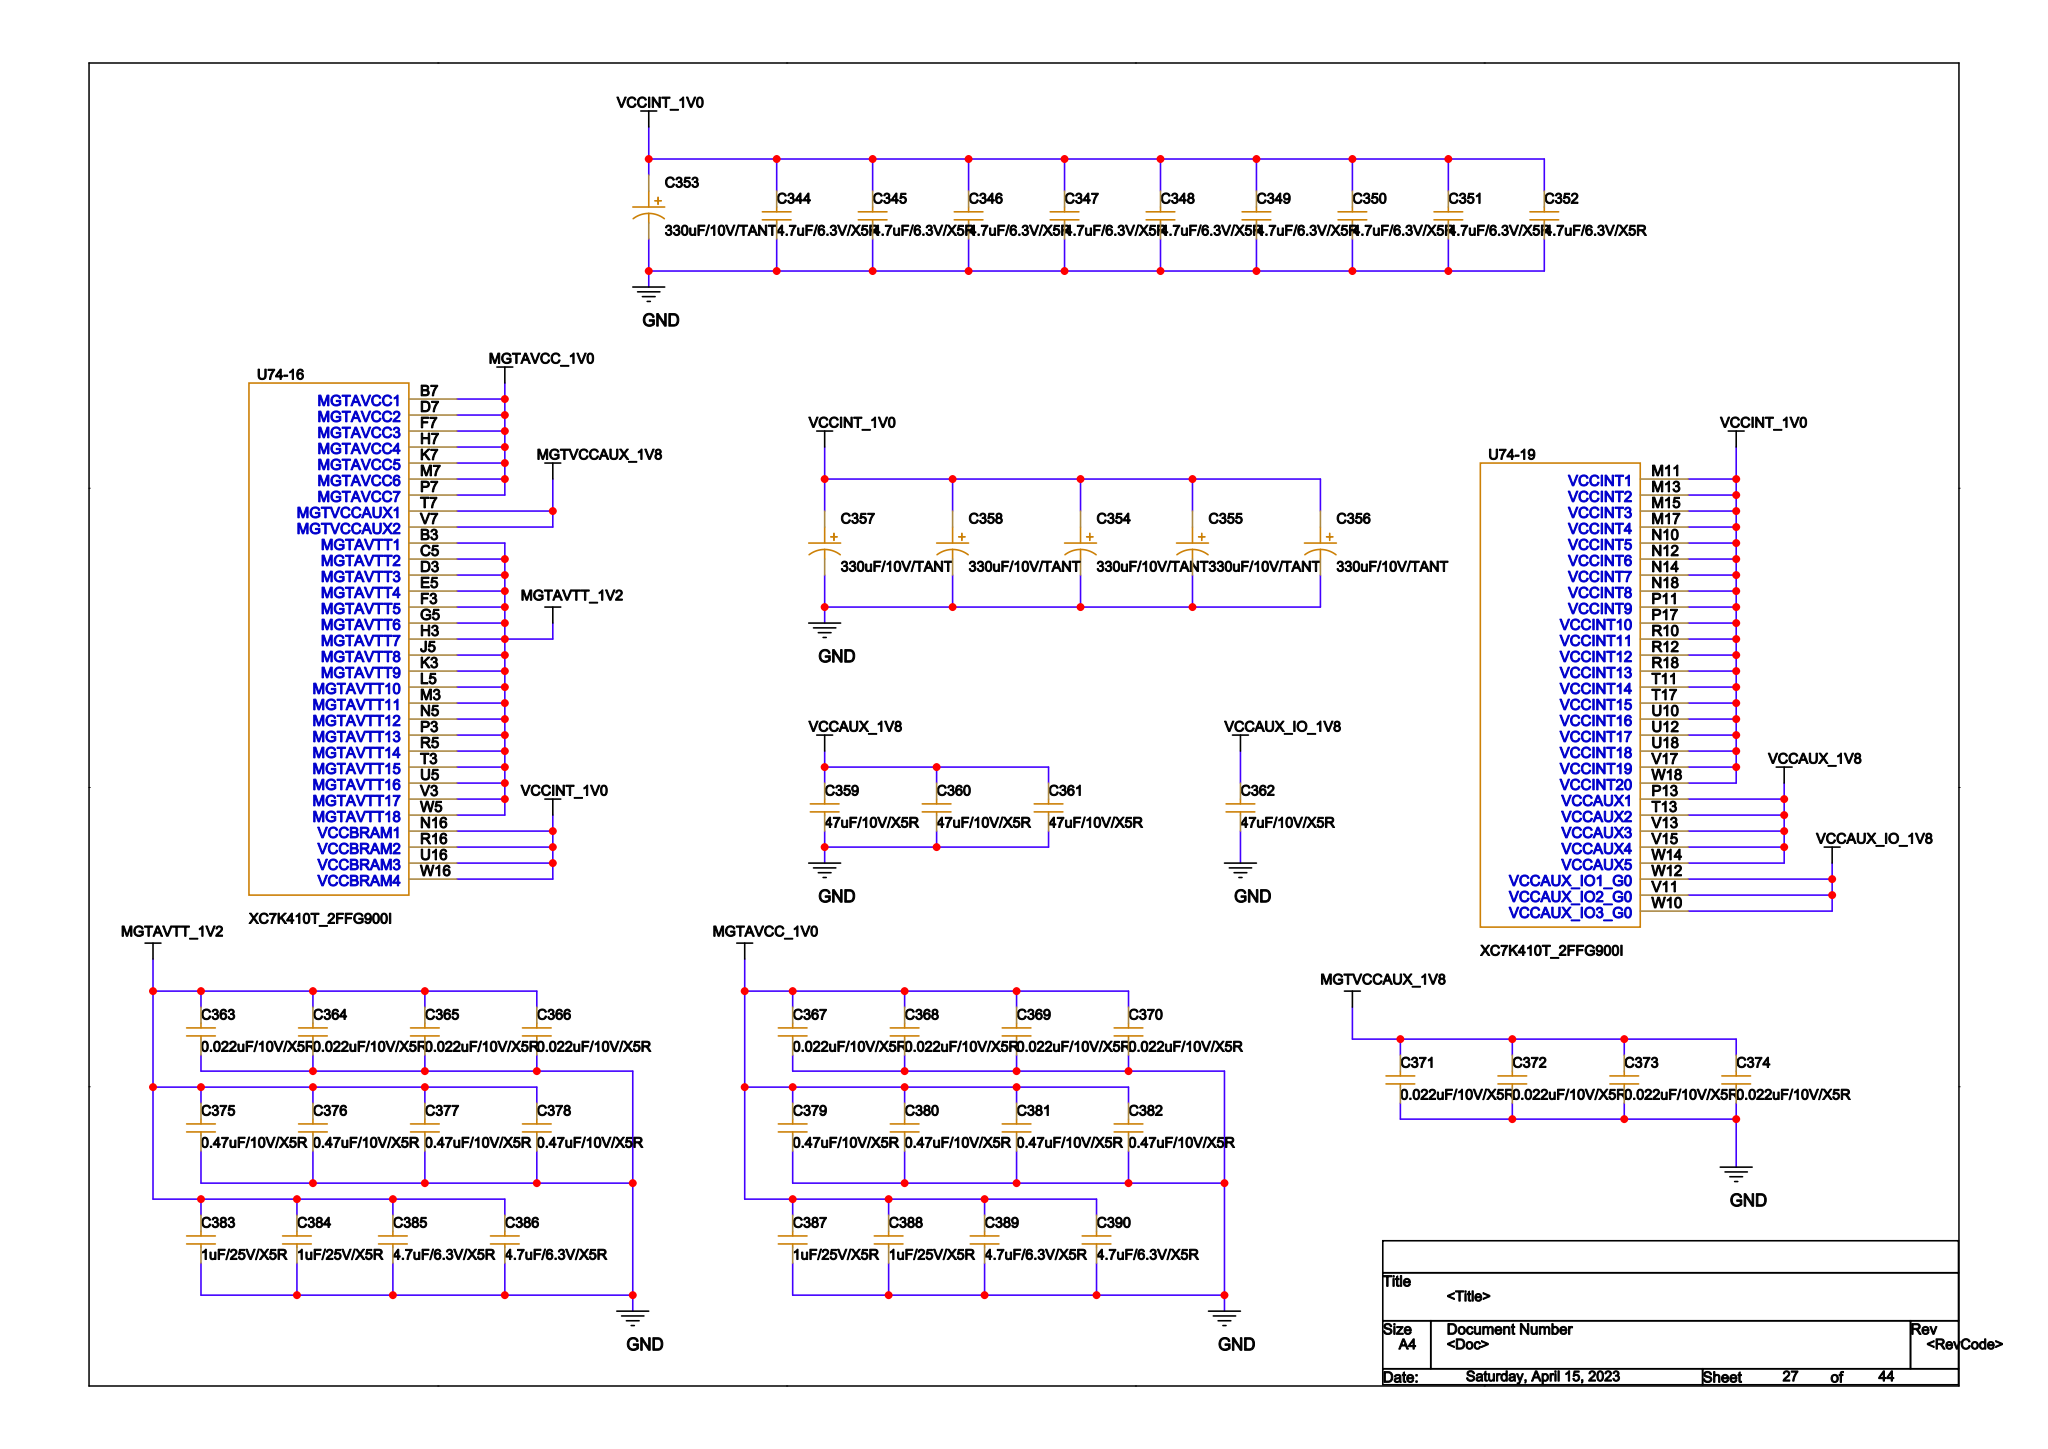Circuit board | Cadence Allegro | 1034 parts | 912 nets | one sheet of the schematic
Parts on this sheet (reference | value | footprint):
C344 | 4.7uF/6.3V/X5R | C0402_BGA
C345 | 4.7uF/6.3V/X5R | C0402_BGA
C346 | 4.7uF/6.3V/X5R | C0402_BGA
C347 | 4.7uF/6.3V/X5R | C0402_BGA
C348 | 4.7uF/6.3V/X5R | C0402_BGA
C349 | 4.7uF/6.3V/X5R | C0402_BGA
C350 | 4.7uF/6.3V/X5R | C0402_BGA
C351 | 4.7uF/6.3V/X5R | C0402_BGA
C352 | 4.7uF/6.3V/X5R | C0402_BGA
C353 | 330uF/10V/TANT | C0402_BGA
C354 | 330uF/10V/TANT | C0402_BGA
C355 | 330uF/10V/TANT | C0402_BGA
C356 | 330uF/10V/TANT | C0402_BGA
C357 | 330uF/10V/TANT | C0402_BGA
C358 | 330uF/10V/TANT | C0402_BGA
C359 | 47uF/10V/X5R | C0402_BGA
C360 | 47uF/10V/X5R | C0402_BGA
C361 | 47uF/10V/X5R | C0402_BGA
C362 | 47uF/10V/X5R | C0402_BGA
C363 | 0.022uF/10V/X5R | C0402_BGA
C364 | 0.022uF/10V/X5R | C0402_BGA
C365 | 0.022uF/10V/X5R | C0402_BGA
C366 | 0.022uF/10V/X5R | C0402_BGA
C367 | 0.022uF/10V/X5R | C0402_BGA
C368 | 0.022uF/10V/X5R | C0402_BGA
C369 | 0.022uF/10V/X5R | C0402_BGA
C370 | 0.022uF/10V/X5R | C0402_BGA
C371 | 0.022uF/10V/X5R | C0402_BGA
C372 | 0.022uF/10V/X5R | C0402_BGA
C373 | 0.022uF/10V/X5R | C0402_BGA
C374 | 0.022uF/10V/X5R | C0402_BGA
C375 | 0.47uF/10V/X5R | C0402_BGA
C376 | 0.47uF/10V/X5R | C0402_BGA
C377 | 0.47uF/10V/X5R | C0402_BGA
C378 | 0.47uF/10V/X5R | C0402_BGA
C379 | 0.47uF/10V/X5R | C0402_BGA
C380 | 0.47uF/10V/X5R | C0402_BGA
C381 | 0.47uF/10V/X5R | C0402_BGA
C382 | 0.47uF/10V/X5R | C0402_BGA
C383 | 1uF/25V/X5R | C0402_BGA
C384 | 1uF/25V/X5R | C0402_BGA
C385 | 4.7uF/6.3V/X5R | C0402_BGA
C386 | 4.7uF/6.3V/X5R | C0402_BGA
C387 | 1uF/25V/X5R | C0402_BGA
C388 | 1uF/25V/X5R | C0402_BGA
C389 | 4.7uF/6.3V/X5R | C0402_BGA
C390 | 4.7uF/6.3V/X5R | C0402_BGA
P3 | TSW-120-07-G-D | TSW_2MM54_DR
Nets of these parts (net: part-pin ...):
GND: C344-1 C345-1 C346-1 C347-1 C348-1 C349-1 C350-1 C351-1 C352-1 C353-2 C354-2 C355-2 C356-2 C357-2 C358-2 C359-1 C360-1 C361-1 C362-1 C363-1 C364-1 C365-1 C366-1 C367-1 C368-1 C369-1 C370-1 C371-1 C372-1 C373-1 C374-1 C375-1 C376-1 C377-1 C378-1 C379-1 C380-1 C381-1 C382-1 C383-1 C384-1 C385-1 C386-1 C387-1 C388-1 C389-1 C390-1 P3-15 P3-27
VCCAUX_1V8: C359-2 C360-2 C361-2
VCCAUX_IO_1V8: C362-2
VCCINT_1V0: C344-2 C345-2 C346-2 C347-2 C348-2 C349-2 C350-2 C351-2 C352-2 C353-1 C354-1 C355-1 C356-1 C357-1 C358-1
MGTAVTT_1V2: C363-2 C364-2 C365-2 C366-2 C375-2 C376-2 C377-2 C378-2 C383-2 C384-2 C385-2 C386-2
MGTAVCC_1V0: C367-2 C368-2 C369-2 C370-2 C379-2 C380-2 C381-2 C382-2 C387-2 C388-2 C389-2 C390-2
MGTVCCAUX_1V8: C371-2 C372-2 C373-2 C374-2